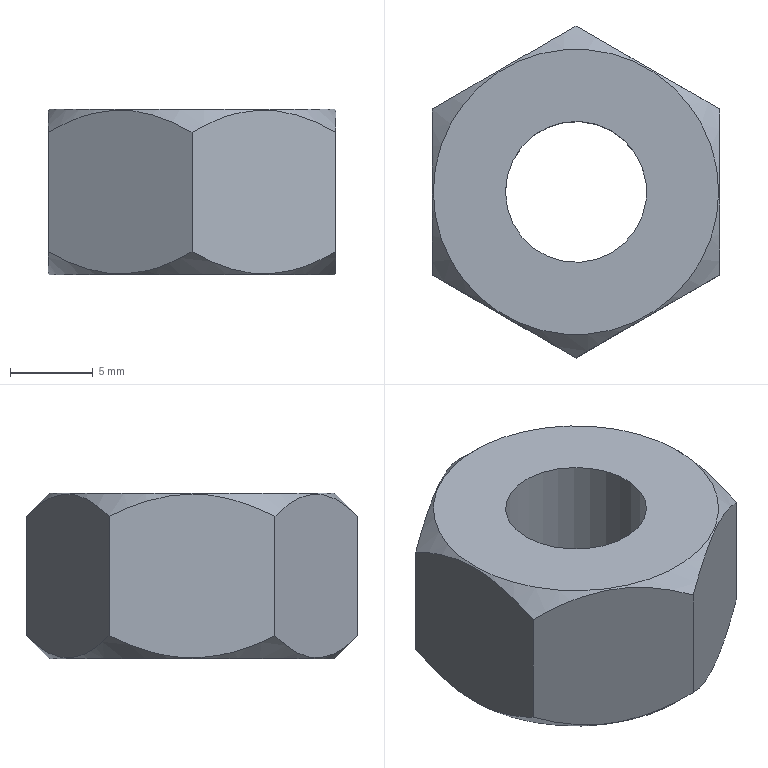Part | NX | features DATUM_CSYS 4, SKETCH 3, EXTRACT_STRING 2, SWP104 2, DATUM_PLANE 1, EXTRUDE 1, HOLE PACKAGE 1, Instance Feature 1, Mirror Feature 1, SIMPLE HOLE 1, SYMBOLIC_THREAD 1 | 1 solid | 11 faces | box 17.321 x 20 x 10 mm | volume 2008 mm3 | plane 8 | cone 2 | cylinder 1 | commonest cylinder face diameters 8.5 x1
STEP:
#1=CARTESIAN_POINT('',(8.66,5.,1.4));
#2=VERTEX_POINT('',#1);
#3=CARTESIAN_POINT('',(8.66,-5.,1.4));
#4=VERTEX_POINT('',#3);
#5=CARTESIAN_POINT('',(8.66,-5.,1.4));
#6=CARTESIAN_POINT('',(8.66,-3.449,0.6243));
#7=CARTESIAN_POINT('',(8.66,0.002747,-0.5048));
#8=CARTESIAN_POINT('',(8.66,3.453,0.6264));
#9=CARTESIAN_POINT('',(8.66,5.,1.4));
#10=B_SPLINE_CURVE_WITH_KNOTS('',3,(#5,#6,#7,#8,#9),.UNSPECIFIED.,.F.,.F.,(4,1,4),(0.006464,0.01165,0.01683),.UNSPECIFIED.);
#11=EDGE_CURVE('',#2,#4,#10,.F.);
#12=ORIENTED_EDGE('',*,*,#11,.F.);
#13=CARTESIAN_POINT('',(8.66,5.,8.6));
#14=VERTEX_POINT('',#13);
#15=CARTESIAN_POINT('',(8.66,5.,10.));
#16=DIRECTION('',(0.,0.,-1.));
#17=VECTOR('',#16,1000.);
#18=LINE('',#15,#17);
#19=EDGE_CURVE('',#14,#2,#18,.T.);
#20=ORIENTED_EDGE('',*,*,#19,.F.);
#21=CARTESIAN_POINT('',(8.66,-5.,8.6));
#22=VERTEX_POINT('',#21);
#23=CARTESIAN_POINT('',(8.66,-5.,8.6));
#24=CARTESIAN_POINT('',(8.66,-3.449,9.376));
#25=CARTESIAN_POINT('',(8.66,0.002747,10.505));
#26=CARTESIAN_POINT('',(8.66,3.453,9.374));
#27=CARTESIAN_POINT('',(8.66,5.,8.6));
#28=B_SPLINE_CURVE_WITH_KNOTS('',3,(#23,#24,#25,#26,#27),.UNSPECIFIED.,.F.,.F.,(4,1,4),(0.006464,0.01165,0.01683),.UNSPECIFIED.);
#29=EDGE_CURVE('',#22,#14,#28,.T.);
#30=ORIENTED_EDGE('',*,*,#29,.F.);
#31=CARTESIAN_POINT('',(8.66,-5.,10.));
#32=DIRECTION('',(0.,0.,-1.));
#33=VECTOR('',#32,1000.);
#34=LINE('',#31,#33);
#35=EDGE_CURVE('',#22,#4,#34,.T.);
#36=ORIENTED_EDGE('',*,*,#35,.T.);
#37=EDGE_LOOP('',(#12,#20,#30,#36));
#38=FACE_BOUND('',#37,.T.);
#39=CARTESIAN_POINT('',(8.66,5.,10.));
#40=DIRECTION('',(1.,0.,0.));
#41=DIRECTION('',(0.,0.,-1.));
#42=AXIS2_PLACEMENT_3D('',#39,#40,#41);
#43=PLANE('',#42);
#44=ADVANCED_FACE('',(#38),#43,.T.);
#45=CARTESIAN_POINT('',(0.,-10.,1.4));
#46=VERTEX_POINT('',#45);
#47=CARTESIAN_POINT('',(8.66,-5.,1.4));
#48=CARTESIAN_POINT('',(7.984,-5.391,1.009));
#49=CARTESIAN_POINT('',(6.61,-6.184,0.3443));
#50=CARTESIAN_POINT('',(3.585,-7.93,-0.2209));
#51=CARTESIAN_POINT('',(1.361,-9.214,0.6141));
#52=CARTESIAN_POINT('',(0.,-10.,1.4));
#53=B_SPLINE_CURVE_WITH_KNOTS('',3,(#47,#48,#49,#50,#51,#52),.UNSPECIFIED.,.F.,.F.,(4,1,1,4),(0.000000254,0.002583,0.005165,0.01033),.UNSPECIFIED.);
#54=EDGE_CURVE('',#4,#46,#53,.T.);
#55=ORIENTED_EDGE('',*,*,#54,.F.);
#56=ORIENTED_EDGE('',*,*,#35,.F.);
#57=CARTESIAN_POINT('',(0.,-10.,8.6));
#58=VERTEX_POINT('',#57);
#59=CARTESIAN_POINT('',(0.,-10.,8.6));
#60=CARTESIAN_POINT('',(0.6766,-9.609,8.991));
#61=CARTESIAN_POINT('',(2.051,-8.816,9.656));
#62=CARTESIAN_POINT('',(5.075,-7.07,10.221));
#63=CARTESIAN_POINT('',(7.299,-5.786,9.386));
#64=CARTESIAN_POINT('',(8.66,-5.,8.6));
#65=B_SPLINE_CURVE_WITH_KNOTS('',3,(#59,#60,#61,#62,#63,#64),.UNSPECIFIED.,.F.,.F.,(4,1,1,4),(0.000000254,0.002583,0.005165,0.01033),.UNSPECIFIED.);
#66=EDGE_CURVE('',#58,#22,#65,.T.);
#67=ORIENTED_EDGE('',*,*,#66,.F.);
#68=CARTESIAN_POINT('',(0.,-10.,10.));
#69=DIRECTION('',(0.,0.,-1.));
#70=VECTOR('',#69,1000.);
#71=LINE('',#68,#70);
#72=EDGE_CURVE('',#58,#46,#71,.T.);
#73=ORIENTED_EDGE('',*,*,#72,.T.);
#74=EDGE_LOOP('',(#55,#56,#67,#73));
#75=FACE_BOUND('',#74,.T.);
#76=CARTESIAN_POINT('',(8.66,-5.,10.));
#77=DIRECTION('',(0.5,-0.866,0.));
#78=DIRECTION('',(0.866,0.5,0.));
#79=AXIS2_PLACEMENT_3D('',#76,#77,#78);
#80=PLANE('',#79);
#81=ADVANCED_FACE('',(#75),#80,.T.);
#82=CARTESIAN_POINT('',(-8.66,-5.,1.4));
#83=VERTEX_POINT('',#82);
#84=CARTESIAN_POINT('',(0.,-10.,1.4));
#85=CARTESIAN_POINT('',(-0.6766,-9.609,1.009));
#86=CARTESIAN_POINT('',(-2.051,-8.816,0.3443));
#87=CARTESIAN_POINT('',(-5.075,-7.07,-0.2209));
#88=CARTESIAN_POINT('',(-7.299,-5.786,0.6141));
#89=CARTESIAN_POINT('',(-8.66,-5.,1.4));
#90=B_SPLINE_CURVE_WITH_KNOTS('',3,(#84,#85,#86,#87,#88,#89),.UNSPECIFIED.,.F.,.F.,(4,1,1,4),(0.000000254,0.002583,0.005165,0.01033),.UNSPECIFIED.);
#91=EDGE_CURVE('',#46,#83,#90,.T.);
#92=ORIENTED_EDGE('',*,*,#91,.F.);
#93=ORIENTED_EDGE('',*,*,#72,.F.);
#94=CARTESIAN_POINT('',(-8.66,-5.,8.6));
#95=VERTEX_POINT('',#94);
#96=CARTESIAN_POINT('',(-8.66,-5.,8.6));
#97=CARTESIAN_POINT('',(-7.984,-5.391,8.991));
#98=CARTESIAN_POINT('',(-6.61,-6.184,9.656));
#99=CARTESIAN_POINT('',(-3.585,-7.93,10.221));
#100=CARTESIAN_POINT('',(-1.361,-9.214,9.386));
#101=CARTESIAN_POINT('',(0.,-10.,8.6));
#102=B_SPLINE_CURVE_WITH_KNOTS('',3,(#96,#97,#98,#99,#100,#101),.UNSPECIFIED.,.F.,.F.,(4,1,1,4),(0.000000254,0.002583,0.005165,0.01033),.UNSPECIFIED.);
#103=EDGE_CURVE('',#95,#58,#102,.T.);
#104=ORIENTED_EDGE('',*,*,#103,.F.);
#105=CARTESIAN_POINT('',(-8.66,-5.,10.));
#106=DIRECTION('',(0.,0.,-1.));
#107=VECTOR('',#106,1000.);
#108=LINE('',#105,#107);
#109=EDGE_CURVE('',#95,#83,#108,.T.);
#110=ORIENTED_EDGE('',*,*,#109,.T.);
#111=EDGE_LOOP('',(#92,#93,#104,#110));
#112=FACE_BOUND('',#111,.T.);
#113=CARTESIAN_POINT('',(0.,-10.,10.));
#114=DIRECTION('',(-0.5,-0.866,0.));
#115=DIRECTION('',(0.866,-0.5,0.));
#116=AXIS2_PLACEMENT_3D('',#113,#114,#115);
#117=PLANE('',#116);
#118=ADVANCED_FACE('',(#112),#117,.T.);
#119=CARTESIAN_POINT('',(-8.66,5.,1.4));
#120=VERTEX_POINT('',#119);
#121=CARTESIAN_POINT('',(-8.66,-5.,1.4));
#122=CARTESIAN_POINT('',(-8.66,-3.449,0.6243));
#123=CARTESIAN_POINT('',(-8.66,0.002747,-0.5048));
#124=CARTESIAN_POINT('',(-8.66,3.453,0.6264));
#125=CARTESIAN_POINT('',(-8.66,5.,1.4));
#126=B_SPLINE_CURVE_WITH_KNOTS('',3,(#121,#122,#123,#124,#125),.UNSPECIFIED.,.F.,.F.,(4,1,4),(0.006464,0.01165,0.01683),.UNSPECIFIED.);
#127=EDGE_CURVE('',#83,#120,#126,.T.);
#128=ORIENTED_EDGE('',*,*,#127,.F.);
#129=ORIENTED_EDGE('',*,*,#109,.F.);
#130=CARTESIAN_POINT('',(-8.66,5.,8.6));
#131=VERTEX_POINT('',#130);
#132=CARTESIAN_POINT('',(-8.66,-5.,8.6));
#133=CARTESIAN_POINT('',(-8.66,-3.449,9.376));
#134=CARTESIAN_POINT('',(-8.66,0.002747,10.505));
#135=CARTESIAN_POINT('',(-8.66,3.453,9.374));
#136=CARTESIAN_POINT('',(-8.66,5.,8.6));
#137=B_SPLINE_CURVE_WITH_KNOTS('',3,(#132,#133,#134,#135,#136),.UNSPECIFIED.,.F.,.F.,(4,1,4),(0.006464,0.01165,0.01683),.UNSPECIFIED.);
#138=EDGE_CURVE('',#131,#95,#137,.F.);
#139=ORIENTED_EDGE('',*,*,#138,.F.);
#140=CARTESIAN_POINT('',(-8.66,5.,10.));
#141=DIRECTION('',(0.,0.,-1.));
#142=VECTOR('',#141,1000.);
#143=LINE('',#140,#142);
#144=EDGE_CURVE('',#131,#120,#143,.T.);
#145=ORIENTED_EDGE('',*,*,#144,.T.);
#146=EDGE_LOOP('',(#128,#129,#139,#145));
#147=FACE_BOUND('',#146,.T.);
#148=CARTESIAN_POINT('',(-8.66,-5.,10.));
#149=DIRECTION('',(-1.,0.,0.));
#150=DIRECTION('',(0.,0.,1.));
#151=AXIS2_PLACEMENT_3D('',#148,#149,#150);
#152=PLANE('',#151);
#153=ADVANCED_FACE('',(#147),#152,.T.);
#154=CARTESIAN_POINT('',(0.,10.,1.4));
#155=VERTEX_POINT('',#154);
#156=CARTESIAN_POINT('',(-8.66,5.,1.4));
#157=CARTESIAN_POINT('',(-7.984,5.391,1.009));
#158=CARTESIAN_POINT('',(-6.61,6.184,0.3443));
#159=CARTESIAN_POINT('',(-3.585,7.93,-0.2209));
#160=CARTESIAN_POINT('',(-1.361,9.214,0.6141));
#161=CARTESIAN_POINT('',(0.,10.,1.4));
#162=B_SPLINE_CURVE_WITH_KNOTS('',3,(#156,#157,#158,#159,#160,#161),.UNSPECIFIED.,.F.,.F.,(4,1,1,4),(0.000000254,0.002583,0.005165,0.01033),.UNSPECIFIED.);
#163=EDGE_CURVE('',#120,#155,#162,.T.);
#164=ORIENTED_EDGE('',*,*,#163,.F.);
#165=ORIENTED_EDGE('',*,*,#144,.F.);
#166=CARTESIAN_POINT('',(0.,10.,8.6));
#167=VERTEX_POINT('',#166);
#168=CARTESIAN_POINT('',(0.,10.,8.6));
#169=CARTESIAN_POINT('',(-0.6766,9.609,8.991));
#170=CARTESIAN_POINT('',(-2.051,8.816,9.656));
#171=CARTESIAN_POINT('',(-5.075,7.07,10.221));
#172=CARTESIAN_POINT('',(-7.299,5.786,9.386));
#173=CARTESIAN_POINT('',(-8.66,5.,8.6));
#174=B_SPLINE_CURVE_WITH_KNOTS('',3,(#168,#169,#170,#171,#172,#173),.UNSPECIFIED.,.F.,.F.,(4,1,1,4),(0.000000254,0.002583,0.005165,0.01033),.UNSPECIFIED.);
#175=EDGE_CURVE('',#167,#131,#174,.T.);
#176=ORIENTED_EDGE('',*,*,#175,.F.);
#177=CARTESIAN_POINT('',(0.,10.,10.));
#178=DIRECTION('',(0.,0.,-1.));
#179=VECTOR('',#178,1000.);
#180=LINE('',#177,#179);
#181=EDGE_CURVE('',#167,#155,#180,.T.);
#182=ORIENTED_EDGE('',*,*,#181,.T.);
#183=EDGE_LOOP('',(#164,#165,#176,#182));
#184=FACE_BOUND('',#183,.T.);
#185=CARTESIAN_POINT('',(-8.66,5.,10.));
#186=DIRECTION('',(-0.5,0.866,0.));
#187=DIRECTION('',(-0.866,-0.5,0.));
#188=AXIS2_PLACEMENT_3D('',#185,#186,#187);
#189=PLANE('',#188);
#190=ADVANCED_FACE('',(#184),#189,.T.);
#191=CARTESIAN_POINT('',(0.,10.,1.4));
#192=CARTESIAN_POINT('',(0.6766,9.609,1.009));
#193=CARTESIAN_POINT('',(2.051,8.816,0.3443));
#194=CARTESIAN_POINT('',(5.075,7.07,-0.2209));
#195=CARTESIAN_POINT('',(7.299,5.786,0.6141));
#196=CARTESIAN_POINT('',(8.66,5.,1.4));
#197=B_SPLINE_CURVE_WITH_KNOTS('',3,(#191,#192,#193,#194,#195,#196),.UNSPECIFIED.,.F.,.F.,(4,1,1,4),(0.000000254,0.002583,0.005165,0.01033),.UNSPECIFIED.);
#198=EDGE_CURVE('',#155,#2,#197,.T.);
#199=ORIENTED_EDGE('',*,*,#198,.F.);
#200=ORIENTED_EDGE('',*,*,#181,.F.);
#201=CARTESIAN_POINT('',(8.66,5.,8.6));
#202=CARTESIAN_POINT('',(7.984,5.391,8.991));
#203=CARTESIAN_POINT('',(6.61,6.184,9.656));
#204=CARTESIAN_POINT('',(3.585,7.93,10.221));
#205=CARTESIAN_POINT('',(1.361,9.214,9.386));
#206=CARTESIAN_POINT('',(0.,10.,8.6));
#207=B_SPLINE_CURVE_WITH_KNOTS('',3,(#201,#202,#203,#204,#205,#206),.UNSPECIFIED.,.F.,.F.,(4,1,1,4),(0.000000254,0.002583,0.005165,0.01033),.UNSPECIFIED.);
#208=EDGE_CURVE('',#14,#167,#207,.T.);
#209=ORIENTED_EDGE('',*,*,#208,.F.);
#210=ORIENTED_EDGE('',*,*,#19,.T.);
#211=EDGE_LOOP('',(#199,#200,#209,#210));
#212=FACE_BOUND('',#211,.T.);
#213=CARTESIAN_POINT('',(0.,10.,10.));
#214=DIRECTION('',(0.5,0.866,0.));
#215=DIRECTION('',(-0.866,0.5,0.));
#216=AXIS2_PLACEMENT_3D('',#213,#214,#215);
#217=PLANE('',#216);
#218=ADVANCED_FACE('',(#212),#217,.T.);
#219=ORIENTED_EDGE('',*,*,#29,.T.);
#220=ORIENTED_EDGE('',*,*,#208,.T.);
#221=ORIENTED_EDGE('',*,*,#175,.T.);
#222=ORIENTED_EDGE('',*,*,#138,.T.);
#223=ORIENTED_EDGE('',*,*,#103,.T.);
#224=ORIENTED_EDGE('',*,*,#66,.T.);
#225=EDGE_LOOP('',(#219,#220,#221,#222,#223,#224));
#226=FACE_BOUND('',#225,.T.);
#227=CARTESIAN_POINT('',(-8.6,0.,10.));
#228=VERTEX_POINT('',#227);
#229=CARTESIAN_POINT('',(0.,0.,10.));
#230=DIRECTION('',(0.,0.,-1.));
#231=DIRECTION('',(-1.,0.,0.));
#232=AXIS2_PLACEMENT_3D('',#229,#230,#231);
#233=CIRCLE('',#232,8.6);
#234=EDGE_CURVE('',#228,#228,#233,.T.);
#235=ORIENTED_EDGE('',*,*,#234,.T.);
#236=EDGE_LOOP('',(#235));
#237=FACE_BOUND('',#236,.T.);
#238=CARTESIAN_POINT('',(0.,0.,10.));
#239=DIRECTION('',(0.,0.,-1.));
#240=DIRECTION('',(-1.,0.,0.));
#241=AXIS2_PLACEMENT_3D('',#238,#239,#240);
#242=CONICAL_SURFACE('',#241,8.6,0.7854);
#243=ADVANCED_FACE('',(#226,#237),#242,.T.);
#244=CARTESIAN_POINT('',(-4.25,0.,10.));
#245=VERTEX_POINT('',#244);
#246=CARTESIAN_POINT('',(0.,0.,10.));
#247=DIRECTION('',(0.,0.,-1.));
#248=DIRECTION('',(-1.,0.,0.));
#249=AXIS2_PLACEMENT_3D('',#246,#247,#248);
#250=CIRCLE('',#249,4.25);
#251=EDGE_CURVE('',#245,#245,#250,.T.);
#252=ORIENTED_EDGE('',*,*,#251,.T.);
#253=EDGE_LOOP('',(#252));
#254=FACE_BOUND('',#253,.T.);
#255=ORIENTED_EDGE('',*,*,#234,.F.);
#256=EDGE_LOOP('',(#255));
#257=FACE_BOUND('',#256,.T.);
#258=CARTESIAN_POINT('',(0.,0.,10.));
#259=DIRECTION('',(0.,0.,-1.));
#260=DIRECTION('',(-1.,0.,0.));
#261=AXIS2_PLACEMENT_3D('',#258,#259,#260);
#262=PLANE('',#261);
#263=ADVANCED_FACE('',(#254,#257),#262,.F.);
#264=ORIENTED_EDGE('',*,*,#11,.T.);
#265=ORIENTED_EDGE('',*,*,#54,.T.);
#266=ORIENTED_EDGE('',*,*,#91,.T.);
#267=ORIENTED_EDGE('',*,*,#127,.T.);
#268=ORIENTED_EDGE('',*,*,#163,.T.);
#269=ORIENTED_EDGE('',*,*,#198,.T.);
#270=EDGE_LOOP('',(#264,#265,#266,#267,#268,#269));
#271=FACE_BOUND('',#270,.T.);
#272=CARTESIAN_POINT('',(8.6,0.,0.));
#273=VERTEX_POINT('',#272);
#274=CARTESIAN_POINT('',(0.,0.,0.));
#275=DIRECTION('',(0.,0.,1.));
#276=DIRECTION('',(1.,0.,0.));
#277=AXIS2_PLACEMENT_3D('',#274,#275,#276);
#278=CIRCLE('',#277,8.6);
#279=EDGE_CURVE('',#273,#273,#278,.T.);
#280=ORIENTED_EDGE('',*,*,#279,.T.);
#281=EDGE_LOOP('',(#280));
#282=FACE_BOUND('',#281,.T.);
#283=CARTESIAN_POINT('',(0.,0.,0.));
#284=DIRECTION('',(0.,0.,1.));
#285=DIRECTION('',(1.,0.,0.));
#286=AXIS2_PLACEMENT_3D('',#283,#284,#285);
#287=CONICAL_SURFACE('',#286,8.6,0.7854);
#288=ADVANCED_FACE('',(#271,#282),#287,.T.);
#289=CARTESIAN_POINT('',(-4.25,0.,0.));
#290=VERTEX_POINT('',#289);
#291=CARTESIAN_POINT('',(0.,0.,0.));
#292=DIRECTION('',(0.,0.,-1.));
#293=DIRECTION('',(-1.,0.,0.));
#294=AXIS2_PLACEMENT_3D('',#291,#292,#293);
#295=CIRCLE('',#294,4.25);
#296=EDGE_CURVE('',#290,#290,#295,.T.);
#297=ORIENTED_EDGE('',*,*,#296,.F.);
#298=EDGE_LOOP('',(#297));
#299=FACE_BOUND('',#298,.T.);
#300=ORIENTED_EDGE('',*,*,#279,.F.);
#301=EDGE_LOOP('',(#300));
#302=FACE_BOUND('',#301,.T.);
#303=CARTESIAN_POINT('',(0.,0.,0.));
#304=DIRECTION('',(0.,0.,-1.));
#305=DIRECTION('',(-1.,0.,0.));
#306=AXIS2_PLACEMENT_3D('',#303,#304,#305);
#307=PLANE('',#306);
#308=ADVANCED_FACE('',(#299,#302),#307,.T.);
#309=ORIENTED_EDGE('',*,*,#296,.T.);
#310=EDGE_LOOP('',(#309));
#311=FACE_BOUND('',#310,.T.);
#312=ORIENTED_EDGE('',*,*,#251,.F.);
#313=EDGE_LOOP('',(#312));
#314=FACE_BOUND('',#313,.T.);
#315=CARTESIAN_POINT('',(0.,0.,10.));
#316=DIRECTION('',(0.,0.,-1.));
#317=DIRECTION('',(-1.,0.,0.));
#318=AXIS2_PLACEMENT_3D('',#315,#316,#317);
#319=CYLINDRICAL_SURFACE('',#318,4.25);
#320=ADVANCED_FACE('',(#311,#314),#319,.F.);
#321=CLOSED_SHELL('',(#44,#81,#118,#153,#190,#218,#243,#263,#288,#308,#320));
#322=MANIFOLD_SOLID_BREP('',#321);
#323=(LENGTH_UNIT()NAMED_UNIT(*)SI_UNIT(.MILLI.,.METRE.));
#324=UNCERTAINTY_MEASURE_WITH_UNIT(LENGTH_MEASURE(0.0508),#323,'','');
#325=(NAMED_UNIT(*)PLANE_ANGLE_UNIT()SI_UNIT($,.RADIAN.));
#326=(NAMED_UNIT(*)SI_UNIT($,.STERADIAN.)SOLID_ANGLE_UNIT());
#327=(GEOMETRIC_REPRESENTATION_CONTEXT(3)GLOBAL_UNCERTAINTY_ASSIGNED_CONTEXT((#324))GLOBAL_UNIT_ASSIGNED_CONTEXT((#323,#325,#326))REPRESENTATION_CONTEXT('',''));
#328=ADVANCED_BREP_SHAPE_REPRESENTATION('',(#322),#327);